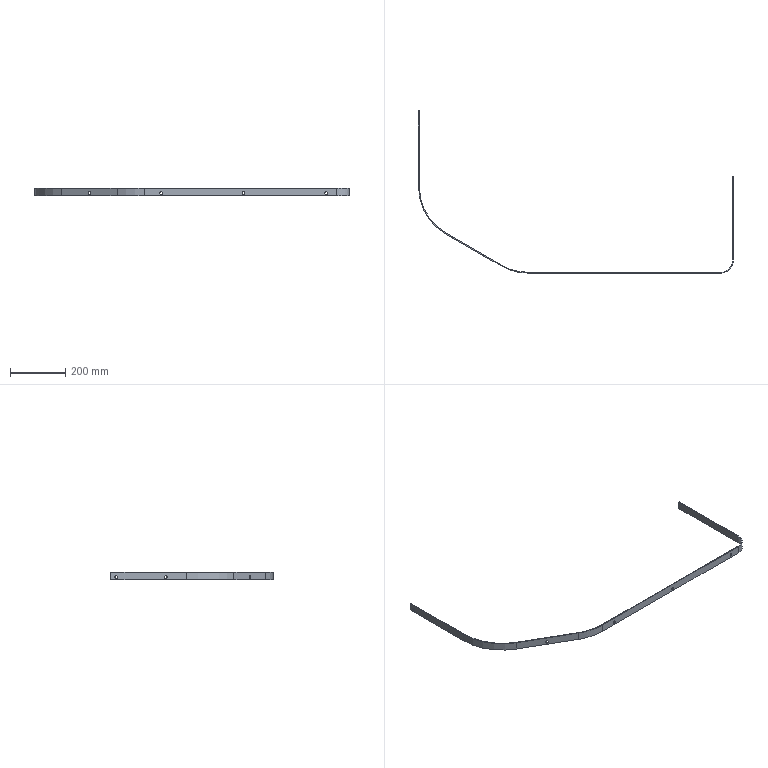Part | SolidWorks | features Cut 2, FlatPattern 1, ICE 1, SMBaseFlange 1, SheetMetal 1 | 1 solid | 42 faces | box 1145 x 590 x 28 mm | volume 157323 mm3 | plane 24 | cylinder 18 | commonest cylinder face diameters 10 x12 390 x2 396 x2 90 x1 96 x1
STEP:
#1=CARTESIAN_POINT('',(-939.643,84.664,-18.));
#2=VERTEX_POINT('',#1);
#3=CARTESIAN_POINT('',(-948.303,89.664,-18.));
#4=VERTEX_POINT('',#3);
#5=CARTESIAN_POINT('',(-943.973,87.164,-18.));
#6=DIRECTION('',(0.5,0.866,0.));
#7=DIRECTION('',(-0.866,0.5,0.));
#8=AXIS2_PLACEMENT_3D('',#5,#6,#7);
#9=CIRCLE('',#8,5.);
#10=EDGE_CURVE('',#2,#4,#9,.T.);
#11=ORIENTED_EDGE('',*,*,#10,.T.);
#12=CARTESIAN_POINT('',(-949.803,87.066,-18.));
#13=VERTEX_POINT('',#12);
#14=CARTESIAN_POINT('',(-944.803,95.726,-18.));
#15=DIRECTION('',(-0.5,-0.866,0.));
#16=VECTOR('',#15,1000.);
#17=LINE('',#14,#16);
#18=EDGE_CURVE('',#4,#13,#17,.T.);
#19=ORIENTED_EDGE('',*,*,#18,.T.);
#20=CARTESIAN_POINT('',(-941.143,82.066,-18.));
#21=VERTEX_POINT('',#20);
#22=CARTESIAN_POINT('',(-945.473,84.566,-18.));
#23=DIRECTION('',(-0.5,-0.866,0.));
#24=DIRECTION('',(0.866,-0.5,0.));
#25=AXIS2_PLACEMENT_3D('',#22,#23,#24);
#26=CIRCLE('',#25,5.);
#27=EDGE_CURVE('',#13,#21,#26,.T.);
#28=ORIENTED_EDGE('',*,*,#27,.T.);
#29=CARTESIAN_POINT('',(-936.143,90.726,-18.));
#30=DIRECTION('',(-0.5,-0.866,0.));
#31=VECTOR('',#30,1000.);
#32=LINE('',#29,#31);
#33=EDGE_CURVE('',#2,#21,#32,.T.);
#34=ORIENTED_EDGE('',*,*,#33,.F.);
#35=EDGE_LOOP('',(#11,#19,#28,#34));
#36=FACE_OUTER_BOUND('',#35,.T.);
#37=CARTESIAN_POINT('',(-940.473,93.226,-18.));
#38=DIRECTION('',(-0.5,-0.866,0.));
#39=DIRECTION('',(0.866,-0.5,0.));
#40=AXIS2_PLACEMENT_3D('',#37,#38,#39);
#41=CYLINDRICAL_SURFACE('',#40,5.);
#42=ADVANCED_FACE('',(#36),#41,.F.);
#43=CARTESIAN_POINT('',(-680.,3.,-18.));
#44=VERTEX_POINT('',#43);
#45=CARTESIAN_POINT('',(-690.,3.,-18.));
#46=VERTEX_POINT('',#45);
#47=CARTESIAN_POINT('',(-685.,3.,-18.));
#48=DIRECTION('',(0.,1.,0.));
#49=DIRECTION('',(-1.,0.,0.));
#50=AXIS2_PLACEMENT_3D('',#47,#48,#49);
#51=CIRCLE('',#50,5.);
#52=EDGE_CURVE('',#44,#46,#51,.T.);
#53=ORIENTED_EDGE('',*,*,#52,.T.);
#54=CARTESIAN_POINT('',(-690.,0.,-18.));
#55=VERTEX_POINT('',#54);
#56=CARTESIAN_POINT('',(-690.,10.,-18.));
#57=DIRECTION('',(0.,-1.,0.));
#58=VECTOR('',#57,1000.);
#59=LINE('',#56,#58);
#60=EDGE_CURVE('',#46,#55,#59,.T.);
#61=ORIENTED_EDGE('',*,*,#60,.T.);
#62=CARTESIAN_POINT('',(-680.,0.,-18.));
#63=VERTEX_POINT('',#62);
#64=CARTESIAN_POINT('',(-685.,0.,-18.));
#65=DIRECTION('',(0.,-1.,0.));
#66=DIRECTION('',(1.,0.,0.));
#67=AXIS2_PLACEMENT_3D('',#64,#65,#66);
#68=CIRCLE('',#67,5.);
#69=EDGE_CURVE('',#55,#63,#68,.T.);
#70=ORIENTED_EDGE('',*,*,#69,.T.);
#71=CARTESIAN_POINT('',(-680.,10.,-18.));
#72=DIRECTION('',(0.,-1.,0.));
#73=VECTOR('',#72,1000.);
#74=LINE('',#71,#73);
#75=EDGE_CURVE('',#44,#63,#74,.T.);
#76=ORIENTED_EDGE('',*,*,#75,.F.);
#77=EDGE_LOOP('',(#53,#61,#70,#76));
#78=FACE_OUTER_BOUND('',#77,.T.);
#79=CARTESIAN_POINT('',(-685.,10.,-18.));
#80=DIRECTION('',(0.,-1.,0.));
#81=DIRECTION('',(1.,0.,0.));
#82=AXIS2_PLACEMENT_3D('',#79,#80,#81);
#83=CYLINDRICAL_SURFACE('',#82,5.);
#84=ADVANCED_FACE('',(#78),#83,.F.);
#85=CARTESIAN_POINT('',(-380.,3.,-18.));
#86=VERTEX_POINT('',#85);
#87=CARTESIAN_POINT('',(-390.,3.,-18.));
#88=VERTEX_POINT('',#87);
#89=CARTESIAN_POINT('',(-385.,3.,-18.));
#90=DIRECTION('',(0.,1.,0.));
#91=DIRECTION('',(-1.,0.,0.));
#92=AXIS2_PLACEMENT_3D('',#89,#90,#91);
#93=CIRCLE('',#92,5.);
#94=EDGE_CURVE('',#86,#88,#93,.T.);
#95=ORIENTED_EDGE('',*,*,#94,.T.);
#96=CARTESIAN_POINT('',(-390.,0.,-18.));
#97=VERTEX_POINT('',#96);
#98=CARTESIAN_POINT('',(-390.,10.,-18.));
#99=DIRECTION('',(0.,-1.,0.));
#100=VECTOR('',#99,1000.);
#101=LINE('',#98,#100);
#102=EDGE_CURVE('',#88,#97,#101,.T.);
#103=ORIENTED_EDGE('',*,*,#102,.T.);
#104=CARTESIAN_POINT('',(-380.,0.,-18.));
#105=VERTEX_POINT('',#104);
#106=CARTESIAN_POINT('',(-385.,0.,-18.));
#107=DIRECTION('',(0.,-1.,0.));
#108=DIRECTION('',(1.,0.,0.));
#109=AXIS2_PLACEMENT_3D('',#106,#107,#108);
#110=CIRCLE('',#109,5.);
#111=EDGE_CURVE('',#97,#105,#110,.T.);
#112=ORIENTED_EDGE('',*,*,#111,.T.);
#113=CARTESIAN_POINT('',(-380.,10.,-18.));
#114=DIRECTION('',(0.,-1.,0.));
#115=VECTOR('',#114,1000.);
#116=LINE('',#113,#115);
#117=EDGE_CURVE('',#86,#105,#116,.T.);
#118=ORIENTED_EDGE('',*,*,#117,.F.);
#119=EDGE_LOOP('',(#95,#103,#112,#118));
#120=FACE_OUTER_BOUND('',#119,.T.);
#121=CARTESIAN_POINT('',(-385.,10.,-18.));
#122=DIRECTION('',(0.,-1.,0.));
#123=DIRECTION('',(1.,0.,0.));
#124=AXIS2_PLACEMENT_3D('',#121,#122,#123);
#125=CYLINDRICAL_SURFACE('',#124,5.);
#126=ADVANCED_FACE('',(#120),#125,.F.);
#127=CARTESIAN_POINT('',(-80.,3.,-18.));
#128=VERTEX_POINT('',#127);
#129=CARTESIAN_POINT('',(-90.,3.,-18.));
#130=VERTEX_POINT('',#129);
#131=CARTESIAN_POINT('',(-85.,3.,-18.));
#132=DIRECTION('',(0.,1.,0.));
#133=DIRECTION('',(-1.,0.,0.));
#134=AXIS2_PLACEMENT_3D('',#131,#132,#133);
#135=CIRCLE('',#134,5.);
#136=EDGE_CURVE('',#128,#130,#135,.T.);
#137=ORIENTED_EDGE('',*,*,#136,.T.);
#138=CARTESIAN_POINT('',(-90.,0.,-18.));
#139=VERTEX_POINT('',#138);
#140=CARTESIAN_POINT('',(-90.,10.,-18.));
#141=DIRECTION('',(0.,-1.,0.));
#142=VECTOR('',#141,1000.);
#143=LINE('',#140,#142);
#144=EDGE_CURVE('',#130,#139,#143,.T.);
#145=ORIENTED_EDGE('',*,*,#144,.T.);
#146=CARTESIAN_POINT('',(-80.,0.,-18.));
#147=VERTEX_POINT('',#146);
#148=CARTESIAN_POINT('',(-85.,0.,-18.));
#149=DIRECTION('',(0.,-1.,0.));
#150=DIRECTION('',(1.,0.,0.));
#151=AXIS2_PLACEMENT_3D('',#148,#149,#150);
#152=CIRCLE('',#151,5.);
#153=EDGE_CURVE('',#139,#147,#152,.T.);
#154=ORIENTED_EDGE('',*,*,#153,.T.);
#155=CARTESIAN_POINT('',(-80.,10.,-18.));
#156=DIRECTION('',(0.,-1.,0.));
#157=VECTOR('',#156,1000.);
#158=LINE('',#155,#157);
#159=EDGE_CURVE('',#128,#147,#158,.T.);
#160=ORIENTED_EDGE('',*,*,#159,.F.);
#161=EDGE_LOOP('',(#137,#145,#154,#160));
#162=FACE_OUTER_BOUND('',#161,.T.);
#163=CARTESIAN_POINT('',(-85.,10.,-18.));
#164=DIRECTION('',(0.,-1.,0.));
#165=DIRECTION('',(1.,0.,0.));
#166=AXIS2_PLACEMENT_3D('',#163,#164,#165);
#167=CYLINDRICAL_SURFACE('',#166,5.);
#168=ADVANCED_FACE('',(#162),#167,.F.);
#169=CARTESIAN_POINT('',(-1142.,570.,-13.));
#170=VERTEX_POINT('',#169);
#171=CARTESIAN_POINT('',(-1142.,570.,-23.));
#172=VERTEX_POINT('',#171);
#173=CARTESIAN_POINT('',(-1142.,570.,-18.));
#174=DIRECTION('',(1.,0.,0.));
#175=DIRECTION('',(0.,0.,-1.));
#176=AXIS2_PLACEMENT_3D('',#173,#174,#175);
#177=CIRCLE('',#176,5.);
#178=EDGE_CURVE('',#170,#172,#177,.T.);
#179=ORIENTED_EDGE('',*,*,#178,.T.);
#180=CARTESIAN_POINT('',(-1145.,570.,-23.));
#181=VERTEX_POINT('',#180);
#182=CARTESIAN_POINT('',(-1135.,570.,-23.));
#183=DIRECTION('',(-1.,0.,0.));
#184=VECTOR('',#183,1000.);
#185=LINE('',#182,#184);
#186=EDGE_CURVE('',#172,#181,#185,.T.);
#187=ORIENTED_EDGE('',*,*,#186,.T.);
#188=CARTESIAN_POINT('',(-1145.,570.,-13.));
#189=VERTEX_POINT('',#188);
#190=CARTESIAN_POINT('',(-1145.,570.,-18.));
#191=DIRECTION('',(-1.,0.,0.));
#192=DIRECTION('',(0.,0.,1.));
#193=AXIS2_PLACEMENT_3D('',#190,#191,#192);
#194=CIRCLE('',#193,5.);
#195=EDGE_CURVE('',#181,#189,#194,.T.);
#196=ORIENTED_EDGE('',*,*,#195,.T.);
#197=CARTESIAN_POINT('',(-1135.,570.,-13.));
#198=DIRECTION('',(-1.,0.,0.));
#199=VECTOR('',#198,1000.);
#200=LINE('',#197,#199);
#201=EDGE_CURVE('',#170,#189,#200,.T.);
#202=ORIENTED_EDGE('',*,*,#201,.F.);
#203=EDGE_LOOP('',(#179,#187,#196,#202));
#204=FACE_OUTER_BOUND('',#203,.T.);
#205=CARTESIAN_POINT('',(-1135.,570.,-18.));
#206=DIRECTION('',(-1.,0.,0.));
#207=DIRECTION('',(0.,0.,1.));
#208=AXIS2_PLACEMENT_3D('',#205,#206,#207);
#209=CYLINDRICAL_SURFACE('',#208,5.);
#210=ADVANCED_FACE('',(#204),#209,.F.);
#211=CARTESIAN_POINT('',(-1142.,390.,-13.));
#212=VERTEX_POINT('',#211);
#213=CARTESIAN_POINT('',(-1142.,390.,-23.));
#214=VERTEX_POINT('',#213);
#215=CARTESIAN_POINT('',(-1142.,390.,-18.));
#216=DIRECTION('',(1.,0.,0.));
#217=DIRECTION('',(0.,0.,-1.));
#218=AXIS2_PLACEMENT_3D('',#215,#216,#217);
#219=CIRCLE('',#218,5.);
#220=EDGE_CURVE('',#212,#214,#219,.T.);
#221=ORIENTED_EDGE('',*,*,#220,.T.);
#222=CARTESIAN_POINT('',(-1145.,390.,-23.));
#223=VERTEX_POINT('',#222);
#224=CARTESIAN_POINT('',(-1135.,390.,-23.));
#225=DIRECTION('',(-1.,0.,0.));
#226=VECTOR('',#225,1000.);
#227=LINE('',#224,#226);
#228=EDGE_CURVE('',#214,#223,#227,.T.);
#229=ORIENTED_EDGE('',*,*,#228,.T.);
#230=CARTESIAN_POINT('',(-1145.,390.,-13.));
#231=VERTEX_POINT('',#230);
#232=CARTESIAN_POINT('',(-1145.,390.,-18.));
#233=DIRECTION('',(-1.,0.,0.));
#234=DIRECTION('',(0.,0.,1.));
#235=AXIS2_PLACEMENT_3D('',#232,#233,#234);
#236=CIRCLE('',#235,5.);
#237=EDGE_CURVE('',#223,#231,#236,.T.);
#238=ORIENTED_EDGE('',*,*,#237,.T.);
#239=CARTESIAN_POINT('',(-1135.,390.,-13.));
#240=DIRECTION('',(-1.,0.,0.));
#241=VECTOR('',#240,1000.);
#242=LINE('',#239,#241);
#243=EDGE_CURVE('',#212,#231,#242,.T.);
#244=ORIENTED_EDGE('',*,*,#243,.F.);
#245=EDGE_LOOP('',(#221,#229,#238,#244));
#246=FACE_OUTER_BOUND('',#245,.T.);
#247=CARTESIAN_POINT('',(-1135.,390.,-18.));
#248=DIRECTION('',(-1.,0.,0.));
#249=DIRECTION('',(0.,0.,1.));
#250=AXIS2_PLACEMENT_3D('',#247,#248,#249);
#251=CYLINDRICAL_SURFACE('',#250,5.);
#252=ADVANCED_FACE('',(#246),#251,.F.);
#253=CARTESIAN_POINT('',(0.,48.,-28.));
#254=VERTEX_POINT('',#253);
#255=CARTESIAN_POINT('',(-3.,48.,-28.));
#256=VERTEX_POINT('',#255);
#257=CARTESIAN_POINT('',(0.,48.,-28.));
#258=DIRECTION('',(-1.,0.,0.));
#259=VECTOR('',#258,1000.);
#260=LINE('',#257,#259);
#261=EDGE_CURVE('',#254,#256,#260,.T.);
#262=ORIENTED_EDGE('',*,*,#261,.F.);
#263=CARTESIAN_POINT('',(-48.,0.,-28.));
#264=VERTEX_POINT('',#263);
#265=CARTESIAN_POINT('',(-48.,48.,-28.));
#266=DIRECTION('',(0.,0.,-1.));
#267=DIRECTION('',(-1.,0.,0.));
#268=AXIS2_PLACEMENT_3D('',#265,#266,#267);
#269=CIRCLE('',#268,48.);
#270=EDGE_CURVE('',#254,#264,#269,.T.);
#271=ORIENTED_EDGE('',*,*,#270,.T.);
#272=CARTESIAN_POINT('',(-48.,3.,-28.));
#273=VERTEX_POINT('',#272);
#274=CARTESIAN_POINT('',(-48.,3.,-28.));
#275=DIRECTION('',(0.,-1.,0.));
#276=VECTOR('',#275,1000.);
#277=LINE('',#274,#276);
#278=EDGE_CURVE('',#273,#264,#277,.T.);
#279=ORIENTED_EDGE('',*,*,#278,.F.);
#280=CARTESIAN_POINT('',(-48.,48.,-28.));
#281=DIRECTION('',(0.,0.,-1.));
#282=DIRECTION('',(1.,0.,0.));
#283=AXIS2_PLACEMENT_3D('',#280,#281,#282);
#284=CIRCLE('',#283,45.);
#285=EDGE_CURVE('',#256,#273,#284,.T.);
#286=ORIENTED_EDGE('',*,*,#285,.F.);
#287=EDGE_LOOP('',(#262,#271,#279,#286));
#288=FACE_OUTER_BOUND('',#287,.T.);
#289=CARTESIAN_POINT('',(0.,48.,-28.));
#290=DIRECTION('',(0.,0.,-1.));
#291=DIRECTION('',(-1.,0.,0.));
#292=AXIS2_PLACEMENT_3D('',#289,#290,#291);
#293=PLANE('',#292);
#294=ADVANCED_FACE('',(#288),#293,.T.);
#295=CARTESIAN_POINT('',(0.,350.,-28.));
#296=VERTEX_POINT('',#295);
#297=CARTESIAN_POINT('',(0.,48.,-28.));
#298=DIRECTION('',(0.,-1.,0.));
#299=VECTOR('',#298,1000.);
#300=LINE('',#297,#299);
#301=EDGE_CURVE('',#296,#254,#300,.T.);
#302=ORIENTED_EDGE('',*,*,#301,.T.);
#303=ORIENTED_EDGE('',*,*,#261,.T.);
#304=CARTESIAN_POINT('',(-3.,350.,-28.));
#305=VERTEX_POINT('',#304);
#306=CARTESIAN_POINT('',(-3.,48.,-28.));
#307=DIRECTION('',(0.,-1.,0.));
#308=VECTOR('',#307,1000.);
#309=LINE('',#306,#308);
#310=EDGE_CURVE('',#305,#256,#309,.T.);
#311=ORIENTED_EDGE('',*,*,#310,.F.);
#312=CARTESIAN_POINT('',(-3.,350.,-28.));
#313=DIRECTION('',(1.,0.,0.));
#314=VECTOR('',#313,1000.);
#315=LINE('',#312,#314);
#316=EDGE_CURVE('',#305,#296,#315,.T.);
#317=ORIENTED_EDGE('',*,*,#316,.T.);
#318=EDGE_LOOP('',(#302,#303,#311,#317));
#319=FACE_OUTER_BOUND('',#318,.T.);
#320=CARTESIAN_POINT('',(-48.,3.,-28.));
#321=DIRECTION('',(0.,0.,-1.));
#322=DIRECTION('',(-1.,0.,0.));
#323=AXIS2_PLACEMENT_3D('',#320,#321,#322);
#324=PLANE('',#323);
#325=ADVANCED_FACE('',(#319),#324,.T.);
#326=CARTESIAN_POINT('',(-48.,0.,0.));
#327=VERTEX_POINT('',#326);
#328=CARTESIAN_POINT('',(-48.,3.,0.));
#329=VERTEX_POINT('',#328);
#330=CARTESIAN_POINT('',(-48.,0.,0.));
#331=DIRECTION('',(0.,1.,0.));
#332=VECTOR('',#331,1000.);
#333=LINE('',#330,#332);
#334=EDGE_CURVE('',#327,#329,#333,.T.);
#335=ORIENTED_EDGE('',*,*,#334,.F.);
#336=CARTESIAN_POINT('',(0.,48.,0.));
#337=VERTEX_POINT('',#336);
#338=CARTESIAN_POINT('',(-48.,48.,0.));
#339=DIRECTION('',(0.,0.,-1.));
#340=DIRECTION('',(-1.,0.,0.));
#341=AXIS2_PLACEMENT_3D('',#338,#339,#340);
#342=CIRCLE('',#341,48.);
#343=EDGE_CURVE('',#337,#327,#342,.T.);
#344=ORIENTED_EDGE('',*,*,#343,.F.);
#345=CARTESIAN_POINT('',(-3.,48.,0.));
#346=VERTEX_POINT('',#345);
#347=CARTESIAN_POINT('',(-3.,48.,0.));
#348=DIRECTION('',(1.,0.,0.));
#349=VECTOR('',#348,1000.);
#350=LINE('',#347,#349);
#351=EDGE_CURVE('',#346,#337,#350,.T.);
#352=ORIENTED_EDGE('',*,*,#351,.F.);
#353=CARTESIAN_POINT('',(-48.,48.,0.));
#354=DIRECTION('',(0.,0.,-1.));
#355=DIRECTION('',(1.,0.,0.));
#356=AXIS2_PLACEMENT_3D('',#353,#354,#355);
#357=CIRCLE('',#356,45.);
#358=EDGE_CURVE('',#346,#329,#357,.T.);
#359=ORIENTED_EDGE('',*,*,#358,.T.);
#360=EDGE_LOOP('',(#335,#344,#352,#359));
#361=FACE_OUTER_BOUND('',#360,.T.);
#362=CARTESIAN_POINT('',(-48.,0.,0.));
#363=DIRECTION('',(0.,0.,1.));
#364=DIRECTION('',(1.,0.,0.));
#365=AXIS2_PLACEMENT_3D('',#362,#363,#364);
#366=PLANE('',#365);
#367=ADVANCED_FACE('',(#361),#366,.T.);
#368=CARTESIAN_POINT('',(-745.946,0.,0.));
#369=VERTEX_POINT('',#368);
#370=CARTESIAN_POINT('',(-48.,0.,0.));
#371=DIRECTION('',(-1.,0.,0.));
#372=VECTOR('',#371,1000.);
#373=LINE('',#370,#372);
#374=EDGE_CURVE('',#327,#369,#373,.T.);
#375=ORIENTED_EDGE('',*,*,#374,.F.);
#376=ORIENTED_EDGE('',*,*,#334,.T.);
#377=CARTESIAN_POINT('',(-745.946,3.,0.));
#378=VERTEX_POINT('',#377);
#379=CARTESIAN_POINT('',(-48.,3.,0.));
#380=DIRECTION('',(-1.,0.,0.));
#381=VECTOR('',#380,1000.);
#382=LINE('',#379,#381);
#383=EDGE_CURVE('',#329,#378,#382,.T.);
#384=ORIENTED_EDGE('',*,*,#383,.T.);
#385=CARTESIAN_POINT('',(-745.946,3.,0.));
#386=DIRECTION('',(0.,-1.,0.));
#387=VECTOR('',#386,1000.);
#388=LINE('',#385,#387);
#389=EDGE_CURVE('',#378,#369,#388,.T.);
#390=ORIENTED_EDGE('',*,*,#389,.T.);
#391=EDGE_LOOP('',(#375,#376,#384,#390));
#392=FACE_OUTER_BOUND('',#391,.T.);
#393=CARTESIAN_POINT('',(-3.,48.,0.));
#394=DIRECTION('',(0.,0.,1.));
#395=DIRECTION('',(1.,0.,0.));
#396=AXIS2_PLACEMENT_3D('',#393,#394,#395);
#397=PLANE('',#396);
#398=ADVANCED_FACE('',(#392),#397,.T.);
#399=CARTESIAN_POINT('',(-745.946,0.,-28.));
#400=VERTEX_POINT('',#399);
#401=CARTESIAN_POINT('',(-745.946,3.,-28.));
#402=VERTEX_POINT('',#401);
#403=CARTESIAN_POINT('',(-745.946,0.,-28.));
#404=DIRECTION('',(0.,1.,0.));
#405=VECTOR('',#404,1000.);
#406=LINE('',#403,#405);
#407=EDGE_CURVE('',#400,#402,#406,.T.);
#408=ORIENTED_EDGE('',*,*,#407,.F.);
#409=CARTESIAN_POINT('',(-844.946,26.527,-28.));
#410=VERTEX_POINT('',#409);
#411=CARTESIAN_POINT('',(-745.946,198.,-28.));
#412=DIRECTION('',(0.,0.,-1.));
#413=DIRECTION('',(-1.,0.,0.));
#414=AXIS2_PLACEMENT_3D('',#411,#412,#413);
#415=CIRCLE('',#414,198.);
#416=EDGE_CURVE('',#400,#410,#415,.T.);
#417=ORIENTED_EDGE('',*,*,#416,.T.);
#418=CARTESIAN_POINT('',(-843.446,29.125,-28.));
#419=VERTEX_POINT('',#418);
#420=CARTESIAN_POINT('',(-843.446,29.125,-28.));
#421=DIRECTION('',(-0.5,-0.866,0.));
#422=VECTOR('',#421,1000.);
#423=LINE('',#420,#422);
#424=EDGE_CURVE('',#419,#410,#423,.T.);
#425=ORIENTED_EDGE('',*,*,#424,.F.);
#426=CARTESIAN_POINT('',(-745.946,198.,-28.));
#427=DIRECTION('',(0.,0.,-1.));
#428=DIRECTION('',(1.,0.,0.));
#429=AXIS2_PLACEMENT_3D('',#426,#427,#428);
#430=CIRCLE('',#429,195.);
#431=EDGE_CURVE('',#402,#419,#430,.T.);
#432=ORIENTED_EDGE('',*,*,#431,.F.);
#433=EDGE_LOOP('',(#408,#417,#425,#432));
#434=FACE_OUTER_BOUND('',#433,.T.);
#435=CARTESIAN_POINT('',(-745.946,0.,-28.));
#436=DIRECTION('',(0.,0.,-1.));
#437=DIRECTION('',(-1.,0.,0.));
#438=AXIS2_PLACEMENT_3D('',#435,#436,#437);
#439=PLANE('',#438);
#440=ADVANCED_FACE('',(#434),#439,.T.);
#441=CARTESIAN_POINT('',(-48.,0.,-28.));
#442=DIRECTION('',(-1.,0.,0.));
#443=VECTOR('',#442,1000.);
#444=LINE('',#441,#443);
#445=EDGE_CURVE('',#264,#400,#444,.T.);
#446=ORIENTED_EDGE('',*,*,#445,.T.);
#447=ORIENTED_EDGE('',*,*,#407,.T.);
#448=CARTESIAN_POINT('',(-48.,3.,-28.));
#449=DIRECTION('',(-1.,0.,0.));
#450=VECTOR('',#449,1000.);
#451=LINE('',#448,#450);
#452=EDGE_CURVE('',#273,#402,#451,.T.);
#453=ORIENTED_EDGE('',*,*,#452,.F.);
#454=ORIENTED_EDGE('',*,*,#278,.T.);
#455=EDGE_LOOP('',(#446,#447,#453,#454));
#456=FACE_OUTER_BOUND('',#455,.T.);
#457=CARTESIAN_POINT('',(-843.446,29.125,-28.));
#458=DIRECTION('',(0.,0.,-1.));
#459=DIRECTION('',(-1.,0.,0.));
#460=AXIS2_PLACEMENT_3D('',#457,#458,#459);
#461=PLANE('',#460);
#462=ADVANCED_FACE('',(#456),#461,.T.);
#463=CARTESIAN_POINT('',(-844.946,26.527,0.));
#464=VERTEX_POINT('',#463);
#465=CARTESIAN_POINT('',(-843.446,29.125,0.));
#466=VERTEX_POINT('',#465);
#467=CARTESIAN_POINT('',(-844.946,26.527,0.));
#468=DIRECTION('',(0.5,0.866,0.));
#469=VECTOR('',#468,1000.);
#470=LINE('',#467,#469);
#471=EDGE_CURVE('',#464,#466,#470,.T.);
#472=ORIENTED_EDGE('',*,*,#471,.F.);
#473=CARTESIAN_POINT('',(-745.946,198.,0.));
#474=DIRECTION('',(0.,0.,-1.));
#475=DIRECTION('',(-1.,0.,0.));
#476=AXIS2_PLACEMENT_3D('',#473,#474,#475);
#477=CIRCLE('',#476,198.);
#478=EDGE_CURVE('',#369,#464,#477,.T.);
#479=ORIENTED_EDGE('',*,*,#478,.F.);
#480=ORIENTED_EDGE('',*,*,#389,.F.);
#481=CARTESIAN_POINT('',(-745.946,198.,0.));
#482=DIRECTION('',(0.,0.,-1.));
#483=DIRECTION('',(1.,0.,0.));
#484=AXIS2_PLACEMENT_3D('',#481,#482,#483);
#485=CIRCLE('',#484,195.);
#486=EDGE_CURVE('',#378,#466,#485,.T.);
#487=ORIENTED_EDGE('',*,*,#486,.T.);
#488=EDGE_LOOP('',(#472,#479,#480,#487));
#489=FACE_OUTER_BOUND('',#488,.T.);
#490=CARTESIAN_POINT('',(-844.946,26.527,0.));
#491=DIRECTION('',(0.,0.,1.));
#492=DIRECTION('',(1.,0.,0.));
#493=AXIS2_PLACEMENT_3D('',#490,#491,#492);
#494=PLANE('',#493);
#495=ADVANCED_FACE('',(#489),#494,.T.);
#496=CARTESIAN_POINT('',(-1046.,142.606,0.));
#497=VERTEX_POINT('',#496);
#498=CARTESIAN_POINT('',(-844.946,26.527,0.));
#499=DIRECTION('',(-0.866,0.5,0.));
#500=VECTOR('',#499,1000.);
#501=LINE('',#498,#500);
#502=EDGE_CURVE('',#464,#497,#501,.T.);
#503=ORIENTED_EDGE('',*,*,#502,.F.);
#504=ORIENTED_EDGE('',*,*,#471,.T.);
#505=CARTESIAN_POINT('',(-1044.5,145.204,0.));
#506=VERTEX_POINT('',#505);
#507=CARTESIAN_POINT('',(-843.446,29.125,0.));
#508=DIRECTION('',(-0.866,0.5,0.));
#509=VECTOR('',#508,1000.);
#510=LINE('',#507,#509);
#511=EDGE_CURVE('',#466,#506,#510,.T.);
#512=ORIENTED_EDGE('',*,*,#511,.T.);
#513=CARTESIAN_POINT('',(-1044.5,145.204,0.));
#514=DIRECTION('',(-0.5,-0.866,0.));
#515=VECTOR('',#514,1000.);
#516=LINE('',#513,#515);
#517=EDGE_CURVE('',#506,#497,#516,.T.);
#518=ORIENTED_EDGE('',*,*,#517,.T.);
#519=EDGE_LOOP('',(#503,#504,#512,#518));
#520=FACE_OUTER_BOUND('',#519,.T.);
#521=CARTESIAN_POINT('',(-745.946,3.,0.));
#522=DIRECTION('',(0.,0.,1.));
#523=DIRECTION('',(1.,0.,0.));
#524=AXIS2_PLACEMENT_3D('',#521,#522,#523);
#525=PLANE('',#524);
#526=ADVANCED_FACE('',(#520),#525,.T.);
#527=CARTESIAN_POINT('',(-1046.,142.606,-28.));
#528=VERTEX_POINT('',#527);
#529=CARTESIAN_POINT('',(-1044.5,145.204,-28.));
#530=VERTEX_POINT('',#529);
#531=CARTESIAN_POINT('',(-1046.,142.606,-28.));
#532=DIRECTION('',(0.5,0.866,0.));
#533=VECTOR('',#532,1000.);
#534=LINE('',#531,#533);
#535=EDGE_CURVE('',#528,#530,#534,.T.);
#536=ORIENTED_EDGE('',*,*,#535,.F.);
#537=CARTESIAN_POINT('',(-1145.,314.079,-28.));
#538=VERTEX_POINT('',#537);
#539=CARTESIAN_POINT('',(-947.,314.079,-28.));
#540=DIRECTION('',(0.,0.,-1.));
#541=DIRECTION('',(1.,0.,0.));
#542=AXIS2_PLACEMENT_3D('',#539,#540,#541);
#543=CIRCLE('',#542,198.);
#544=EDGE_CURVE('',#528,#538,#543,.T.);
#545=ORIENTED_EDGE('',*,*,#544,.T.);
#546=CARTESIAN_POINT('',(-1142.,314.079,-28.));
#547=VERTEX_POINT('',#546);
#548=CARTESIAN_POINT('',(-1142.,314.079,-28.));
#549=DIRECTION('',(-1.,0.,0.));
#550=VECTOR('',#549,1000.);
#551=LINE('',#548,#550);
#552=EDGE_CURVE('',#547,#538,#551,.T.);
#553=ORIENTED_EDGE('',*,*,#552,.F.);
#554=CARTESIAN_POINT('',(-947.,314.079,-28.));
#555=DIRECTION('',(0.,0.,-1.));
#556=DIRECTION('',(1.,0.,0.));
#557=AXIS2_PLACEMENT_3D('',#554,#555,#556);
#558=CIRCLE('',#557,195.);
#559=EDGE_CURVE('',#530,#547,#558,.T.);
#560=ORIENTED_EDGE('',*,*,#559,.F.);
#561=EDGE_LOOP('',(#536,#545,#553,#560));
#562=FACE_OUTER_BOUND('',#561,.T.);
#563=CARTESIAN_POINT('',(-1046.,142.606,-28.));
#564=DIRECTION('',(0.,0.,-1.));
#565=DIRECTION('',(-1.,0.,0.));
#566=AXIS2_PLACEMENT_3D('',#563,#564,#565);
#567=PLANE('',#566);
#568=ADVANCED_FACE('',(#562),#567,.T.);
#569=CARTESIAN_POINT('',(-844.946,26.527,-28.));
#570=DIRECTION('',(-0.866,0.5,0.));
#571=VECTOR('',#570,1000.);
#572=LINE('',#569,#571);
#573=EDGE_CURVE('',#410,#528,#572,.T.);
#574=ORIENTED_EDGE('',*,*,#573,.T.);
#575=ORIENTED_EDGE('',*,*,#535,.T.);
#576=CARTESIAN_POINT('',(-843.446,29.125,-28.));
#577=DIRECTION('',(-0.866,0.5,0.));
#578=VECTOR('',#577,1000.);
#579=LINE('',#576,#578);
#580=EDGE_CURVE('',#419,#530,#579,.T.);
#581=ORIENTED_EDGE('',*,*,#580,.F.);
#582=ORIENTED_EDGE('',*,*,#424,.T.);
#583=EDGE_LOOP('',(#574,#575,#581,#582));
#584=FACE_OUTER_BOUND('',#583,.T.);
#585=CARTESIAN_POINT('',(-1142.,314.079,-28.));
#586=DIRECTION('',(0.,0.,-1.));
#587=DIRECTION('',(-1.,0.,0.));
#588=AXIS2_PLACEMENT_3D('',#585,#586,#587);
#589=PLANE('',#588);
#590=ADVANCED_FACE('',(#584),#589,.T.);
#591=CARTESIAN_POINT('',(-1145.,314.079,0.));
#592=VERTEX_POINT('',#591);
#593=CARTESIAN_POINT('',(-1142.,314.079,0.));
#594=VERTEX_POINT('',#593);
#595=CARTESIAN_POINT('',(-1145.,314.079,0.));
#596=DIRECTION('',(1.,0.,0.));
#597=VECTOR('',#596,1000.);
#598=LINE('',#595,#597);
#599=EDGE_CURVE('',#592,#594,#598,.T.);
#600=ORIENTED_EDGE('',*,*,#599,.F.);
#601=CARTESIAN_POINT('',(-947.,314.079,0.));
#602=DIRECTION('',(0.,0.,-1.));
#603=DIRECTION('',(1.,0.,0.));
#604=AXIS2_PLACEMENT_3D('',#601,#602,#603);
#605=CIRCLE('',#604,198.);
#606=EDGE_CURVE('',#497,#592,#605,.T.);
#607=ORIENTED_EDGE('',*,*,#606,.F.);
#608=ORIENTED_EDGE('',*,*,#517,.F.);
#609=CARTESIAN_POINT('',(-947.,314.079,0.));
#610=DIRECTION('',(0.,0.,-1.));
#611=DIRECTION('',(1.,0.,0.));
#612=AXIS2_PLACEMENT_3D('',#609,#610,#611);
#613=CIRCLE('',#612,195.);
#614=EDGE_CURVE('',#506,#594,#613,.T.);
#615=ORIENTED_EDGE('',*,*,#614,.T.);
#616=EDGE_LOOP('',(#600,#607,#608,#615));
#617=FACE_OUTER_BOUND('',#616,.T.);
#618=CARTESIAN_POINT('',(-1145.,314.079,0.));
#619=DIRECTION('',(0.,0.,1.));
#620=DIRECTION('',(1.,0.,0.));
#621=AXIS2_PLACEMENT_3D('',#618,#619,#620);
#622=PLANE('',#621);
#623=ADVANCED_FACE('',(#617),#622,.T.);
#624=CARTESIAN_POINT('',(-1145.,590.,0.));
#625=VERTEX_POINT('',#624);
#626=CARTESIAN_POINT('',(-1145.,314.079,0.));
#627=DIRECTION('',(0.,1.,0.));
#628=VECTOR('',#627,1000.);
#629=LINE('',#626,#628);
#630=EDGE_CURVE('',#592,#625,#629,.T.);
#631=ORIENTED_EDGE('',*,*,#630,.F.);
#632=ORIENTED_EDGE('',*,*,#599,.T.);
#633=CARTESIAN_POINT('',(-1142.,590.,0.));
#634=VERTEX_POINT('',#633);
#635=CARTESIAN_POINT('',(-1142.,314.079,0.));
#636=DIRECTION('',(0.,1.,0.));
#637=VECTOR('',#636,1000.);
#638=LINE('',#635,#637);
#639=EDGE_CURVE('',#594,#634,#638,.T.);
#640=ORIENTED_EDGE('',*,*,#639,.T.);
#641=CARTESIAN_POINT('',(-1145.,590.,0.));
#642=DIRECTION('',(1.,0.,0.));
#643=VECTOR('',#642,1000.);
#644=LINE('',#641,#643);
#645=EDGE_CURVE('',#625,#634,#644,.T.);
#646=ORIENTED_EDGE('',*,*,#645,.F.);
#647=EDGE_LOOP('',(#631,#632,#640,#646));
#648=FACE_OUTER_BOUND('',#647,.T.);
#649=CARTESIAN_POINT('',(-1044.5,145.204,0.));
#650=DIRECTION('',(0.,0.,1.));
#651=DIRECTION('',(1.,0.,0.));
#652=AXIS2_PLACEMENT_3D('',#649,#650,#651);
#653=PLANE('',#652);
#654=ADVANCED_FACE('',(#648),#653,.T.);
#655=ORIENTED_EDGE('',*,*,#178,.F.);
#656=CARTESIAN_POINT('',(-1142.,570.,-18.));
#657=DIRECTION('',(1.,0.,0.));
#658=DIRECTION('',(0.,0.,-1.));
#659=AXIS2_PLACEMENT_3D('',#656,#657,#658);
#660=CIRCLE('',#659,5.);
#661=EDGE_CURVE('',#172,#170,#660,.T.);
#662=ORIENTED_EDGE('',*,*,#661,.F.);
#663=EDGE_LOOP('',(#655,#662));
#664=FACE_BOUND('',#663,.T.);
#665=ORIENTED_EDGE('',*,*,#220,.F.);
#666=CARTESIAN_POINT('',(-1142.,390.,-18.));
#667=DIRECTION('',(1.,0.,0.));
#668=DIRECTION('',(0.,0.,-1.));
#669=AXIS2_PLACEMENT_3D('',#666,#667,#668);
#670=CIRCLE('',#669,5.);
#671=EDGE_CURVE('',#214,#212,#670,.T.);
#672=ORIENTED_EDGE('',*,*,#671,.F.);
#673=EDGE_LOOP('',(#665,#672));
#674=FACE_BOUND('',#673,.T.);
#675=ORIENTED_EDGE('',*,*,#639,.F.);
#676=CARTESIAN_POINT('',(-1142.,314.079,-28.));
#677=DIRECTION('',(0.,0.,1.));
#678=VECTOR('',#677,1000.);
#679=LINE('',#676,#678);
#680=EDGE_CURVE('',#547,#594,#679,.T.);
#681=ORIENTED_EDGE('',*,*,#680,.F.);
#682=CARTESIAN_POINT('',(-1142.,590.,-28.));
#683=VERTEX_POINT('',#682);
#684=CARTESIAN_POINT('',(-1142.,314.079,-28.));
#685=DIRECTION('',(0.,1.,0.));
#686=VECTOR('',#685,1000.);
#687=LINE('',#684,#686);
#688=EDGE_CURVE('',#547,#683,#687,.T.);
#689=ORIENTED_EDGE('',*,*,#688,.T.);
#690=CARTESIAN_POINT('',(-1142.,590.,-28.));
#691=DIRECTION('',(0.,0.,1.));
#692=VECTOR('',#691,1000.);
#693=LINE('',#690,#692);
#694=EDGE_CURVE('',#683,#634,#693,.T.);
#695=ORIENTED_EDGE('',*,*,#694,.T.);
#696=EDGE_LOOP('',(#675,#681,#689,#695));
#697=FACE_OUTER_BOUND('',#696,.T.);
#698=CARTESIAN_POINT('',(-1142.,314.079,-28.));
#699=DIRECTION('',(1.,0.,0.));
#700=DIRECTION('',(0.,0.,-1.));
#701=AXIS2_PLACEMENT_3D('',#698,#699,#700);
#702=PLANE('',#701);
#703=ADVANCED_FACE('',(#664,#674,#697),#702,.T.);
#704=ORIENTED_EDGE('',*,*,#614,.F.);
#705=CARTESIAN_POINT('',(-1044.5,145.204,-28.));
#706=DIRECTION('',(0.,0.,1.));
#707=VECTOR('',#706,1000.);
#708=LINE('',#705,#707);
#709=EDGE_CURVE('',#530,#506,#708,.T.);
#710=ORIENTED_EDGE('',*,*,#709,.F.);
#711=ORIENTED_EDGE('',*,*,#559,.T.);
#712=ORIENTED_EDGE('',*,*,#680,.T.);
#713=EDGE_LOOP('',(#704,#710,#711,#712));
#714=FACE_OUTER_BOUND('',#713,.T.);
#715=CARTESIAN_POINT('',(-947.,314.079,-28.));
#716=DIRECTION('',(0.,0.,1.));
#717=DIRECTION('',(1.,0.,0.));
#718=AXIS2_PLACEMENT_3D('',#715,#716,#717);
#719=CYLINDRICAL_SURFACE('',#718,195.);
#720=ADVANCED_FACE('',(#714),#719,.F.);
#721=ORIENTED_EDGE('',*,*,#10,.F.);
#722=CARTESIAN_POINT('',(-943.973,87.164,-18.));
#723=DIRECTION('',(0.5,0.866,0.));
#724=DIRECTION('',(-0.866,0.5,0.));
#725=AXIS2_PLACEMENT_3D('',#722,#723,#724);
#726=CIRCLE('',#725,5.);
#727=EDGE_CURVE('',#4,#2,#726,.T.);
#728=ORIENTED_EDGE('',*,*,#727,.F.);
#729=EDGE_LOOP('',(#721,#728));
#730=FACE_BOUND('',#729,.T.);
#731=ORIENTED_EDGE('',*,*,#511,.F.);
#732=CARTESIAN_POINT('',(-843.446,29.125,-28.));
#733=DIRECTION('',(0.,0.,1.));
#734=VECTOR('',#733,1000.);
#735=LINE('',#732,#734);
#736=EDGE_CURVE('',#419,#466,#735,.T.);
#737=ORIENTED_EDGE('',*,*,#736,.F.);
#738=ORIENTED_EDGE('',*,*,#580,.T.);
#739=ORIENTED_EDGE('',*,*,#709,.T.);
#740=EDGE_LOOP('',(#731,#737,#738,#739));
#741=FACE_OUTER_BOUND('',#740,.T.);
#742=CARTESIAN_POINT('',(-843.446,29.125,-28.));
#743=DIRECTION('',(0.5,0.866,0.));
#744=DIRECTION('',(-0.866,0.5,0.));
#745=AXIS2_PLACEMENT_3D('',#742,#743,#744);
#746=PLANE('',#745);
#747=ADVANCED_FACE('',(#730,#741),#746,.T.);
#748=ORIENTED_EDGE('',*,*,#486,.F.);
#749=CARTESIAN_POINT('',(-745.946,3.,-28.));
#750=DIRECTION('',(0.,0.,1.));
#751=VECTOR('',#750,1000.);
#752=LINE('',#749,#751);
#753=EDGE_CURVE('',#402,#378,#752,.T.);
#754=ORIENTED_EDGE('',*,*,#753,.F.);
#755=ORIENTED_EDGE('',*,*,#431,.T.);
#756=ORIENTED_EDGE('',*,*,#736,.T.);
#757=EDGE_LOOP('',(#748,#754,#755,#756));
#758=FACE_OUTER_BOUND('',#757,.T.);
#759=CARTESIAN_POINT('',(-745.946,198.,-28.));
#760=DIRECTION('',(0.,0.,1.));
#761=DIRECTION('',(1.,0.,0.));
#762=AXIS2_PLACEMENT_3D('',#759,#760,#761);
#763=CYLINDRICAL_SURFACE('',#762,195.);
#764=ADVANCED_FACE('',(#758),#763,.F.);
#765=ORIENTED_EDGE('',*,*,#52,.F.);
#766=CARTESIAN_POINT('',(-685.,3.,-18.));
#767=DIRECTION('',(0.,1.,0.));
#768=DIRECTION('',(-1.,0.,0.));
#769=AXIS2_PLACEMENT_3D('',#766,#767,#768);
#770=CIRCLE('',#769,5.);
#771=EDGE_CURVE('',#46,#44,#770,.T.);
#772=ORIENTED_EDGE('',*,*,#771,.F.);
#773=EDGE_LOOP('',(#765,#772));
#774=FACE_BOUND('',#773,.T.);
#775=ORIENTED_EDGE('',*,*,#94,.F.);
#776=CARTESIAN_POINT('',(-385.,3.,-18.));
#777=DIRECTION('',(0.,1.,0.));
#778=DIRECTION('',(-1.,0.,0.));
#779=AXIS2_PLACEMENT_3D('',#776,#777,#778);
#780=CIRCLE('',#779,5.);
#781=EDGE_CURVE('',#88,#86,#780,.T.);
#782=ORIENTED_EDGE('',*,*,#781,.F.);
#783=EDGE_LOOP('',(#775,#782));
#784=FACE_BOUND('',#783,.T.);
#785=ORIENTED_EDGE('',*,*,#136,.F.);
#786=CARTESIAN_POINT('',(-85.,3.,-18.));
#787=DIRECTION('',(0.,1.,0.));
#788=DIRECTION('',(-1.,0.,0.));
#789=AXIS2_PLACEMENT_3D('',#786,#787,#788);
#790=CIRCLE('',#789,5.);
#791=EDGE_CURVE('',#130,#128,#790,.T.);
#792=ORIENTED_EDGE('',*,*,#791,.F.);
#793=EDGE_LOOP('',(#785,#792));
#794=FACE_BOUND('',#793,.T.);
#795=ORIENTED_EDGE('',*,*,#383,.F.);
#796=CARTESIAN_POINT('',(-48.,3.,-28.));
#797=DIRECTION('',(0.,0.,1.));
#798=VECTOR('',#797,1000.);
#799=LINE('',#796,#798);
#800=EDGE_CURVE('',#273,#329,#799,.T.);
#801=ORIENTED_EDGE('',*,*,#800,.F.);
#802=ORIENTED_EDGE('',*,*,#452,.T.);
#803=ORIENTED_EDGE('',*,*,#753,.T.);
#804=EDGE_LOOP('',(#795,#801,#802,#803));
#805=FACE_OUTER_BOUND('',#804,.T.);
#806=CARTESIAN_POINT('',(-48.,3.,-28.));
#807=DIRECTION('',(0.,1.,0.));
#808=DIRECTION('',(-1.,0.,0.));
#809=AXIS2_PLACEMENT_3D('',#806,#807,#808);
#810=PLANE('',#809);
#811=ADVANCED_FACE('',(#774,#784,#794,#805),#810,.T.);
#812=ORIENTED_EDGE('',*,*,#358,.F.);
#813=CARTESIAN_POINT('',(-3.,48.,-28.));
#814=DIRECTION('',(0.,0.,1.));
#815=VECTOR('',#814,1000.);
#816=LINE('',#813,#815);
#817=EDGE_CURVE('',#256,#346,#816,.T.);
#818=ORIENTED_EDGE('',*,*,#817,.F.);
#819=ORIENTED_EDGE('',*,*,#285,.T.);
#820=ORIENTED_EDGE('',*,*,#800,.T.);
#821=EDGE_LOOP('',(#812,#818,#819,#820));
#822=FACE_OUTER_BOUND('',#821,.T.);
#823=CARTESIAN_POINT('',(-48.,48.,-28.));
#824=DIRECTION('',(0.,0.,1.));
#825=DIRECTION('',(1.,0.,0.));
#826=AXIS2_PLACEMENT_3D('',#823,#824,#825);
#827=CYLINDRICAL_SURFACE('',#826,45.);
#828=ADVANCED_FACE('',(#822),#827,.F.);
#829=CARTESIAN_POINT('',(-3.,350.,0.));
#830=VERTEX_POINT('',#829);
#831=CARTESIAN_POINT('',(-3.,48.,0.));
#832=DIRECTION('',(0.,-1.,0.));
#833=VECTOR('',#832,1000.);
#834=LINE('',#831,#833);
#835=EDGE_CURVE('',#830,#346,#834,.T.);
#836=ORIENTED_EDGE('',*,*,#835,.F.);
#837=CARTESIAN_POINT('',(-3.,350.,-28.));
#838=DIRECTION('',(0.,0.,1.));
#839=VECTOR('',#838,1000.);
#840=LINE('',#837,#839);
#841=EDGE_CURVE('',#305,#830,#840,.T.);
#842=ORIENTED_EDGE('',*,*,#841,.F.);
#843=ORIENTED_EDGE('',*,*,#310,.T.);
#844=ORIENTED_EDGE('',*,*,#817,.T.);
#845=EDGE_LOOP('',(#836,#842,#843,#844));
#846=FACE_OUTER_BOUND('',#845,.T.);
#847=CARTESIAN_POINT('',(-3.,48.,-28.));
#848=DIRECTION('',(-1.,0.,0.));
#849=DIRECTION('',(0.,0.,1.));
#850=AXIS2_PLACEMENT_3D('',#847,#848,#849);
#851=PLANE('',#850);
#852=ADVANCED_FACE('',(#846),#851,.T.);
#853=CARTESIAN_POINT('',(0.,350.,0.));
#854=VERTEX_POINT('',#853);
#855=CARTESIAN_POINT('',(-3.,350.,0.));
#856=DIRECTION('',(1.,0.,0.));
#857=VECTOR('',#856,1000.);
#858=LINE('',#855,#857);
#859=EDGE_CURVE('',#830,#854,#858,.T.);
#860=ORIENTED_EDGE('',*,*,#859,.T.);
#861=CARTESIAN_POINT('',(0.,350.,-28.));
#862=DIRECTION('',(0.,0.,1.));
#863=VECTOR('',#862,1000.);
#864=LINE('',#861,#863);
#865=EDGE_CURVE('',#296,#854,#864,.T.);
#866=ORIENTED_EDGE('',*,*,#865,.F.);
#867=ORIENTED_EDGE('',*,*,#316,.F.);
#868=ORIENTED_EDGE('',*,*,#841,.T.);
#869=EDGE_LOOP('',(#860,#866,#867,#868));
#870=FACE_OUTER_BOUND('',#869,.T.);
#871=CARTESIAN_POINT('',(-3.,350.,-28.));
#872=DIRECTION('',(0.,-1.,0.));
#873=DIRECTION('',(0.,0.,-1.));
#874=AXIS2_PLACEMENT_3D('',#871,#872,#873);
#875=PLANE('',#874);
#876=ADVANCED_FACE('',(#870),#875,.F.);
#877=CARTESIAN_POINT('',(0.,48.,0.));
#878=DIRECTION('',(0.,-1.,0.));
#879=VECTOR('',#878,1000.);
#880=LINE('',#877,#879);
#881=EDGE_CURVE('',#854,#337,#880,.T.);
#882=ORIENTED_EDGE('',*,*,#881,.T.);
#883=CARTESIAN_POINT('',(0.,48.,-28.));
#884=DIRECTION('',(0.,0.,1.));
#885=VECTOR('',#884,1000.);
#886=LINE('',#883,#885);
#887=EDGE_CURVE('',#254,#337,#886,.T.);
#888=ORIENTED_EDGE('',*,*,#887,.F.);
#889=ORIENTED_EDGE('',*,*,#301,.F.);
#890=ORIENTED_EDGE('',*,*,#865,.T.);
#891=EDGE_LOOP('',(#882,#888,#889,#890));
#892=FACE_OUTER_BOUND('',#891,.T.);
#893=CARTESIAN_POINT('',(0.,48.,-28.));
#894=DIRECTION('',(-1.,0.,0.));
#895=DIRECTION('',(0.,0.,1.));
#896=AXIS2_PLACEMENT_3D('',#893,#894,#895);
#897=PLANE('',#896);
#898=ADVANCED_FACE('',(#892),#897,.F.);
#899=ORIENTED_EDGE('',*,*,#343,.T.);
#900=CARTESIAN_POINT('',(-48.,0.,-28.));
#901=DIRECTION('',(0.,0.,1.));
#902=VECTOR('',#901,1000.);
#903=LINE('',#900,#902);
#904=EDGE_CURVE('',#264,#327,#903,.T.);
#905=ORIENTED_EDGE('',*,*,#904,.F.);
#906=ORIENTED_EDGE('',*,*,#270,.F.);
#907=ORIENTED_EDGE('',*,*,#887,.T.);
#908=EDGE_LOOP('',(#899,#905,#906,#907));
#909=FACE_OUTER_BOUND('',#908,.T.);
#910=CARTESIAN_POINT('',(-48.,48.,-28.));
#911=DIRECTION('',(0.,0.,1.));
#912=DIRECTION('',(1.,0.,0.));
#913=AXIS2_PLACEMENT_3D('',#910,#911,#912);
#914=CYLINDRICAL_SURFACE('',#913,48.);
#915=ADVANCED_FACE('',(#909),#914,.T.);
#916=CARTESIAN_POINT('',(-685.,0.,-18.));
#917=DIRECTION('',(0.,-1.,0.));
#918=DIRECTION('',(1.,0.,0.));
#919=AXIS2_PLACEMENT_3D('',#916,#917,#918);
#920=CIRCLE('',#919,5.);
#921=EDGE_CURVE('',#63,#55,#920,.T.);
#922=ORIENTED_EDGE('',*,*,#921,.F.);
#923=ORIENTED_EDGE('',*,*,#69,.F.);
#924=EDGE_LOOP('',(#922,#923));
#925=FACE_BOUND('',#924,.T.);
#926=CARTESIAN_POINT('',(-385.,0.,-18.));
#927=DIRECTION('',(0.,-1.,0.));
#928=DIRECTION('',(1.,0.,0.));
#929=AXIS2_PLACEMENT_3D('',#926,#927,#928);
#930=CIRCLE('',#929,5.);
#931=EDGE_CURVE('',#105,#97,#930,.T.);
#932=ORIENTED_EDGE('',*,*,#931,.F.);
#933=ORIENTED_EDGE('',*,*,#111,.F.);
#934=EDGE_LOOP('',(#932,#933));
#935=FACE_BOUND('',#934,.T.);
#936=CARTESIAN_POINT('',(-85.,0.,-18.));
#937=DIRECTION('',(0.,-1.,0.));
#938=DIRECTION('',(1.,0.,0.));
#939=AXIS2_PLACEMENT_3D('',#936,#937,#938);
#940=CIRCLE('',#939,5.);
#941=EDGE_CURVE('',#147,#139,#940,.T.);
#942=ORIENTED_EDGE('',*,*,#941,.F.);
#943=ORIENTED_EDGE('',*,*,#153,.F.);
#944=EDGE_LOOP('',(#942,#943));
#945=FACE_BOUND('',#944,.T.);
#946=ORIENTED_EDGE('',*,*,#374,.T.);
#947=CARTESIAN_POINT('',(-745.946,0.,-28.));
#948=DIRECTION('',(0.,0.,1.));
#949=VECTOR('',#948,1000.);
#950=LINE('',#947,#949);
#951=EDGE_CURVE('',#400,#369,#950,.T.);
#952=ORIENTED_EDGE('',*,*,#951,.F.);
#953=ORIENTED_EDGE('',*,*,#445,.F.);
#954=ORIENTED_EDGE('',*,*,#904,.T.);
#955=EDGE_LOOP('',(#946,#952,#953,#954));
#956=FACE_OUTER_BOUND('',#955,.T.);
#957=CARTESIAN_POINT('',(-48.,0.,-28.));
#958=DIRECTION('',(0.,1.,0.));
#959=DIRECTION('',(-1.,0.,0.));
#960=AXIS2_PLACEMENT_3D('',#957,#958,#959);
#961=PLANE('',#960);
#962=ADVANCED_FACE('',(#925,#935,#945,#956),#961,.F.);
#963=ORIENTED_EDGE('',*,*,#478,.T.);
#964=CARTESIAN_POINT('',(-844.946,26.527,-28.));
#965=DIRECTION('',(0.,0.,1.));
#966=VECTOR('',#965,1000.);
#967=LINE('',#964,#966);
#968=EDGE_CURVE('',#410,#464,#967,.T.);
#969=ORIENTED_EDGE('',*,*,#968,.F.);
#970=ORIENTED_EDGE('',*,*,#416,.F.);
#971=ORIENTED_EDGE('',*,*,#951,.T.);
#972=EDGE_LOOP('',(#963,#969,#970,#971));
#973=FACE_OUTER_BOUND('',#972,.T.);
#974=CARTESIAN_POINT('',(-745.946,198.,-28.));
#975=DIRECTION('',(0.,0.,1.));
#976=DIRECTION('',(1.,0.,0.));
#977=AXIS2_PLACEMENT_3D('',#974,#975,#976);
#978=CYLINDRICAL_SURFACE('',#977,198.);
#979=ADVANCED_FACE('',(#973),#978,.T.);
#980=CARTESIAN_POINT('',(-945.473,84.566,-18.));
#981=DIRECTION('',(-0.5,-0.866,0.));
#982=DIRECTION('',(0.866,-0.5,0.));
#983=AXIS2_PLACEMENT_3D('',#980,#981,#982);
#984=CIRCLE('',#983,5.);
#985=EDGE_CURVE('',#21,#13,#984,.T.);
#986=ORIENTED_EDGE('',*,*,#985,.F.);
#987=ORIENTED_EDGE('',*,*,#27,.F.);
#988=EDGE_LOOP('',(#986,#987));
#989=FACE_BOUND('',#988,.T.);
#990=ORIENTED_EDGE('',*,*,#502,.T.);
#991=CARTESIAN_POINT('',(-1046.,142.606,-28.));
#992=DIRECTION('',(0.,0.,1.));
#993=VECTOR('',#992,1000.);
#994=LINE('',#991,#993);
#995=EDGE_CURVE('',#528,#497,#994,.T.);
#996=ORIENTED_EDGE('',*,*,#995,.F.);
#997=ORIENTED_EDGE('',*,*,#573,.F.);
#998=ORIENTED_EDGE('',*,*,#968,.T.);
#999=EDGE_LOOP('',(#990,#996,#997,#998));
#1000=FACE_OUTER_BOUND('',#999,.T.);
#1001=CARTESIAN_POINT('',(-844.946,26.527,-28.));
#1002=DIRECTION('',(0.5,0.866,0.));
#1003=DIRECTION('',(-0.866,0.5,0.));
#1004=AXIS2_PLACEMENT_3D('',#1001,#1002,#1003);
#1005=PLANE('',#1004);
#1006=ADVANCED_FACE('',(#989,#1000),#1005,.F.);
#1007=ORIENTED_EDGE('',*,*,#606,.T.);
#1008=CARTESIAN_POINT('',(-1145.,314.079,-28.));
#1009=DIRECTION('',(0.,0.,1.));
#1010=VECTOR('',#1009,1000.);
#1011=LINE('',#1008,#1010);
#1012=EDGE_CURVE('',#538,#592,#1011,.T.);
#1013=ORIENTED_EDGE('',*,*,#1012,.F.);
#1014=ORIENTED_EDGE('',*,*,#544,.F.);
#1015=ORIENTED_EDGE('',*,*,#995,.T.);
#1016=EDGE_LOOP('',(#1007,#1013,#1014,#1015));
#1017=FACE_OUTER_BOUND('',#1016,.T.);
#1018=CARTESIAN_POINT('',(-947.,314.079,-28.));
#1019=DIRECTION('',(0.,0.,1.));
#1020=DIRECTION('',(1.,0.,0.));
#1021=AXIS2_PLACEMENT_3D('',#1018,#1019,#1020);
#1022=CYLINDRICAL_SURFACE('',#1021,198.);
#1023=ADVANCED_FACE('',(#1017),#1022,.T.);
#1024=CARTESIAN_POINT('',(-1145.,570.,-18.));
#1025=DIRECTION('',(-1.,0.,0.));
#1026=DIRECTION('',(0.,0.,1.));
#1027=AXIS2_PLACEMENT_3D('',#1024,#1025,#1026);
#1028=CIRCLE('',#1027,5.);
#1029=EDGE_CURVE('',#189,#181,#1028,.T.);
#1030=ORIENTED_EDGE('',*,*,#1029,.F.);
#1031=ORIENTED_EDGE('',*,*,#195,.F.);
#1032=EDGE_LOOP('',(#1030,#1031));
#1033=FACE_BOUND('',#1032,.T.);
#1034=CARTESIAN_POINT('',(-1145.,390.,-18.));
#1035=DIRECTION('',(-1.,0.,0.));
#1036=DIRECTION('',(0.,0.,1.));
#1037=AXIS2_PLACEMENT_3D('',#1034,#1035,#1036);
#1038=CIRCLE('',#1037,5.);
#1039=EDGE_CURVE('',#231,#223,#1038,.T.);
#1040=ORIENTED_EDGE('',*,*,#1039,.F.);
#1041=ORIENTED_EDGE('',*,*,#237,.F.);
#1042=EDGE_LOOP('',(#1040,#1041));
#1043=FACE_BOUND('',#1042,.T.);
#1044=ORIENTED_EDGE('',*,*,#630,.T.);
#1045=CARTESIAN_POINT('',(-1145.,590.,-28.));
#1046=VERTEX_POINT('',#1045);
#1047=CARTESIAN_POINT('',(-1145.,590.,-28.));
#1048=DIRECTION('',(0.,0.,1.));
#1049=VECTOR('',#1048,1000.);
#1050=LINE('',#1047,#1049);
#1051=EDGE_CURVE('',#1046,#625,#1050,.T.);
#1052=ORIENTED_EDGE('',*,*,#1051,.F.);
#1053=CARTESIAN_POINT('',(-1145.,314.079,-28.));
#1054=DIRECTION('',(0.,1.,0.));
#1055=VECTOR('',#1054,1000.);
#1056=LINE('',#1053,#1055);
#1057=EDGE_CURVE('',#538,#1046,#1056,.T.);
#1058=ORIENTED_EDGE('',*,*,#1057,.F.);
#1059=ORIENTED_EDGE('',*,*,#1012,.T.);
#1060=EDGE_LOOP('',(#1044,#1052,#1058,#1059));
#1061=FACE_OUTER_BOUND('',#1060,.T.);
#1062=CARTESIAN_POINT('',(-1145.,314.079,-28.));
#1063=DIRECTION('',(1.,0.,0.));
#1064=DIRECTION('',(0.,0.,-1.));
#1065=AXIS2_PLACEMENT_3D('',#1062,#1063,#1064);
#1066=PLANE('',#1065);
#1067=ADVANCED_FACE('',(#1033,#1043,#1061),#1066,.F.);
#1068=ORIENTED_EDGE('',*,*,#645,.T.);
#1069=ORIENTED_EDGE('',*,*,#694,.F.);
#1070=CARTESIAN_POINT('',(-1145.,590.,-28.));
#1071=DIRECTION('',(1.,0.,0.));
#1072=VECTOR('',#1071,1000.);
#1073=LINE('',#1070,#1072);
#1074=EDGE_CURVE('',#1046,#683,#1073,.T.);
#1075=ORIENTED_EDGE('',*,*,#1074,.F.);
#1076=ORIENTED_EDGE('',*,*,#1051,.T.);
#1077=EDGE_LOOP('',(#1068,#1069,#1075,#1076));
#1078=FACE_OUTER_BOUND('',#1077,.T.);
#1079=CARTESIAN_POINT('',(-1145.,590.,-28.));
#1080=DIRECTION('',(0.,-1.,0.));
#1081=DIRECTION('',(0.,0.,-1.));
#1082=AXIS2_PLACEMENT_3D('',#1079,#1080,#1081);
#1083=PLANE('',#1082);
#1084=ADVANCED_FACE('',(#1078),#1083,.F.);
#1085=ORIENTED_EDGE('',*,*,#688,.F.);
#1086=ORIENTED_EDGE('',*,*,#552,.T.);
#1087=ORIENTED_EDGE('',*,*,#1057,.T.);
#1088=ORIENTED_EDGE('',*,*,#1074,.T.);
#1089=EDGE_LOOP('',(#1085,#1086,#1087,#1088));
#1090=FACE_OUTER_BOUND('',#1089,.T.);
#1091=CARTESIAN_POINT('',(-947.,314.079,-28.));
#1092=DIRECTION('',(0.,0.,-1.));
#1093=DIRECTION('',(-1.,0.,0.));
#1094=AXIS2_PLACEMENT_3D('',#1091,#1092,#1093);
#1095=PLANE('',#1094);
#1096=ADVANCED_FACE('',(#1090),#1095,.T.);
#1097=ORIENTED_EDGE('',*,*,#835,.T.);
#1098=ORIENTED_EDGE('',*,*,#351,.T.);
#1099=ORIENTED_EDGE('',*,*,#881,.F.);
#1100=ORIENTED_EDGE('',*,*,#859,.F.);
#1101=EDGE_LOOP('',(#1097,#1098,#1099,#1100));
#1102=FACE_OUTER_BOUND('',#1101,.T.);
#1103=CARTESIAN_POINT('',(-947.,314.079,0.));
#1104=DIRECTION('',(0.,0.,-1.));
#1105=DIRECTION('',(-1.,0.,0.));
#1106=AXIS2_PLACEMENT_3D('',#1103,#1104,#1105);
#1107=PLANE('',#1106);
#1108=ADVANCED_FACE('',(#1102),#1107,.F.);
#1109=ORIENTED_EDGE('',*,*,#228,.F.);
#1110=ORIENTED_EDGE('',*,*,#671,.T.);
#1111=ORIENTED_EDGE('',*,*,#243,.T.);
#1112=ORIENTED_EDGE('',*,*,#1039,.T.);
#1113=EDGE_LOOP('',(#1109,#1110,#1111,#1112));
#1114=FACE_OUTER_BOUND('',#1113,.T.);
#1115=CARTESIAN_POINT('',(-1135.,390.,-18.));
#1116=DIRECTION('',(-1.,0.,0.));
#1117=DIRECTION('',(0.,0.,1.));
#1118=AXIS2_PLACEMENT_3D('',#1115,#1116,#1117);
#1119=CYLINDRICAL_SURFACE('',#1118,5.);
#1120=ADVANCED_FACE('',(#1114),#1119,.F.);
#1121=ORIENTED_EDGE('',*,*,#186,.F.);
#1122=ORIENTED_EDGE('',*,*,#661,.T.);
#1123=ORIENTED_EDGE('',*,*,#201,.T.);
#1124=ORIENTED_EDGE('',*,*,#1029,.T.);
#1125=EDGE_LOOP('',(#1121,#1122,#1123,#1124));
#1126=FACE_OUTER_BOUND('',#1125,.T.);
#1127=CARTESIAN_POINT('',(-1135.,570.,-18.));
#1128=DIRECTION('',(-1.,0.,0.));
#1129=DIRECTION('',(0.,0.,1.));
#1130=AXIS2_PLACEMENT_3D('',#1127,#1128,#1129);
#1131=CYLINDRICAL_SURFACE('',#1130,5.);
#1132=ADVANCED_FACE('',(#1126),#1131,.F.);
#1133=ORIENTED_EDGE('',*,*,#144,.F.);
#1134=ORIENTED_EDGE('',*,*,#791,.T.);
#1135=ORIENTED_EDGE('',*,*,#159,.T.);
#1136=ORIENTED_EDGE('',*,*,#941,.T.);
#1137=EDGE_LOOP('',(#1133,#1134,#1135,#1136));
#1138=FACE_OUTER_BOUND('',#1137,.T.);
#1139=CARTESIAN_POINT('',(-85.,10.,-18.));
#1140=DIRECTION('',(0.,-1.,0.));
#1141=DIRECTION('',(1.,0.,0.));
#1142=AXIS2_PLACEMENT_3D('',#1139,#1140,#1141);
#1143=CYLINDRICAL_SURFACE('',#1142,5.);
#1144=ADVANCED_FACE('',(#1138),#1143,.F.);
#1145=ORIENTED_EDGE('',*,*,#102,.F.);
#1146=ORIENTED_EDGE('',*,*,#781,.T.);
#1147=ORIENTED_EDGE('',*,*,#117,.T.);
#1148=ORIENTED_EDGE('',*,*,#931,.T.);
#1149=EDGE_LOOP('',(#1145,#1146,#1147,#1148));
#1150=FACE_OUTER_BOUND('',#1149,.T.);
#1151=CARTESIAN_POINT('',(-385.,10.,-18.));
#1152=DIRECTION('',(0.,-1.,0.));
#1153=DIRECTION('',(1.,0.,0.));
#1154=AXIS2_PLACEMENT_3D('',#1151,#1152,#1153);
#1155=CYLINDRICAL_SURFACE('',#1154,5.);
#1156=ADVANCED_FACE('',(#1150),#1155,.F.);
#1157=ORIENTED_EDGE('',*,*,#60,.F.);
#1158=ORIENTED_EDGE('',*,*,#771,.T.);
#1159=ORIENTED_EDGE('',*,*,#75,.T.);
#1160=ORIENTED_EDGE('',*,*,#921,.T.);
#1161=EDGE_LOOP('',(#1157,#1158,#1159,#1160));
#1162=FACE_OUTER_BOUND('',#1161,.T.);
#1163=CARTESIAN_POINT('',(-685.,10.,-18.));
#1164=DIRECTION('',(0.,-1.,0.));
#1165=DIRECTION('',(1.,0.,0.));
#1166=AXIS2_PLACEMENT_3D('',#1163,#1164,#1165);
#1167=CYLINDRICAL_SURFACE('',#1166,5.);
#1168=ADVANCED_FACE('',(#1162),#1167,.F.);
#1169=ORIENTED_EDGE('',*,*,#18,.F.);
#1170=ORIENTED_EDGE('',*,*,#727,.T.);
#1171=ORIENTED_EDGE('',*,*,#33,.T.);
#1172=ORIENTED_EDGE('',*,*,#985,.T.);
#1173=EDGE_LOOP('',(#1169,#1170,#1171,#1172));
#1174=FACE_OUTER_BOUND('',#1173,.T.);
#1175=CARTESIAN_POINT('',(-940.473,93.226,-18.));
#1176=DIRECTION('',(-0.5,-0.866,0.));
#1177=DIRECTION('',(0.866,-0.5,0.));
#1178=AXIS2_PLACEMENT_3D('',#1175,#1176,#1177);
#1179=CYLINDRICAL_SURFACE('',#1178,5.);
#1180=ADVANCED_FACE('',(#1174),#1179,.F.);
#1181=CLOSED_SHELL('',(#42,#84,#126,#168,#210,#252,#294,#325,#367,#398,#440,#462,#495,#526,#568,#590,#623,#654,#703,#720,#747,#764,#811,#828,#852,#876,#898,#915,#962,#979,#1006,#1023,#1067,#1084,#1096,#1108,#1120,#1132,#1144,#1156,#1168,#1180));
#1182=MANIFOLD_SOLID_BREP('',#1181);
#1183=CARTESIAN_POINT('',(0.,0.,0.));
#1184=DIRECTION('',(0.,0.,1.));
#1185=DIRECTION('',(1.,0.,0.));
#1186=AXIS2_PLACEMENT_3D('',#1183,#1184,#1185);
#1187=(LENGTH_UNIT()NAMED_UNIT(*)SI_UNIT(.MILLI.,.METRE.));
#1188=UNCERTAINTY_MEASURE_WITH_UNIT(LENGTH_MEASURE(0.00001),#1187,'','');
#1189=(NAMED_UNIT(*)PLANE_ANGLE_UNIT()SI_UNIT($,.RADIAN.));
#1190=(NAMED_UNIT(*)SI_UNIT($,.STERADIAN.)SOLID_ANGLE_UNIT());
#1191=(GEOMETRIC_REPRESENTATION_CONTEXT(3)GLOBAL_UNCERTAINTY_ASSIGNED_CONTEXT((#1188))GLOBAL_UNIT_ASSIGNED_CONTEXT((#1187,#1189,#1190))REPRESENTATION_CONTEXT('',''));
#1192=ADVANCED_BREP_SHAPE_REPRESENTATION('',(#1182,#1186),#1191);